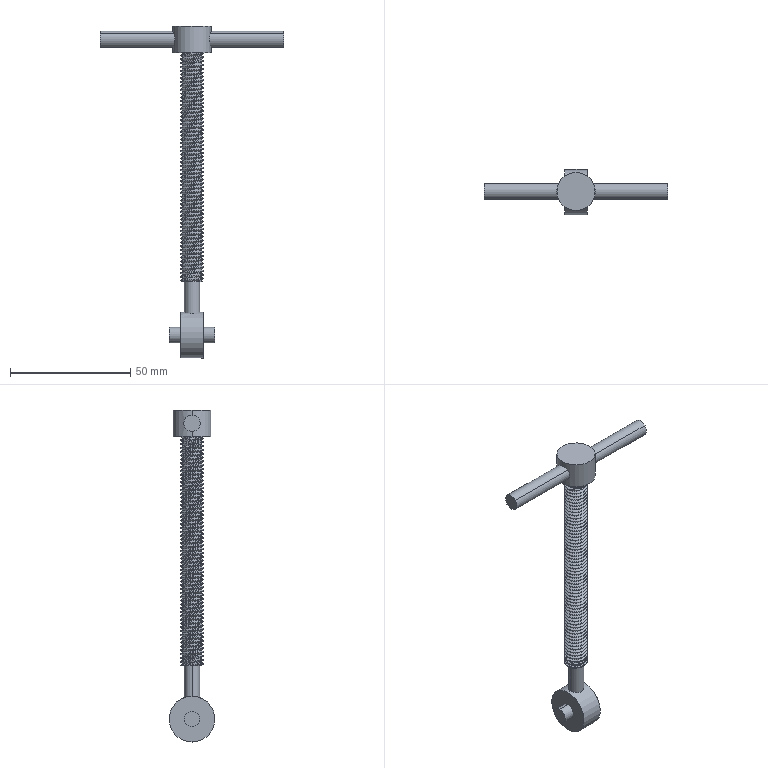Part | SolidWorks | 3 solids | 151 faces | box 76.2 x 19.05 x 138.125 mm | volume 13340 mm3 | cylinder 137 | plane 11 | spline 3 | commonest cylinder face diameters 9.55 x121 6.35 x8 6.756 x4 15.875 x2 19.05 x2